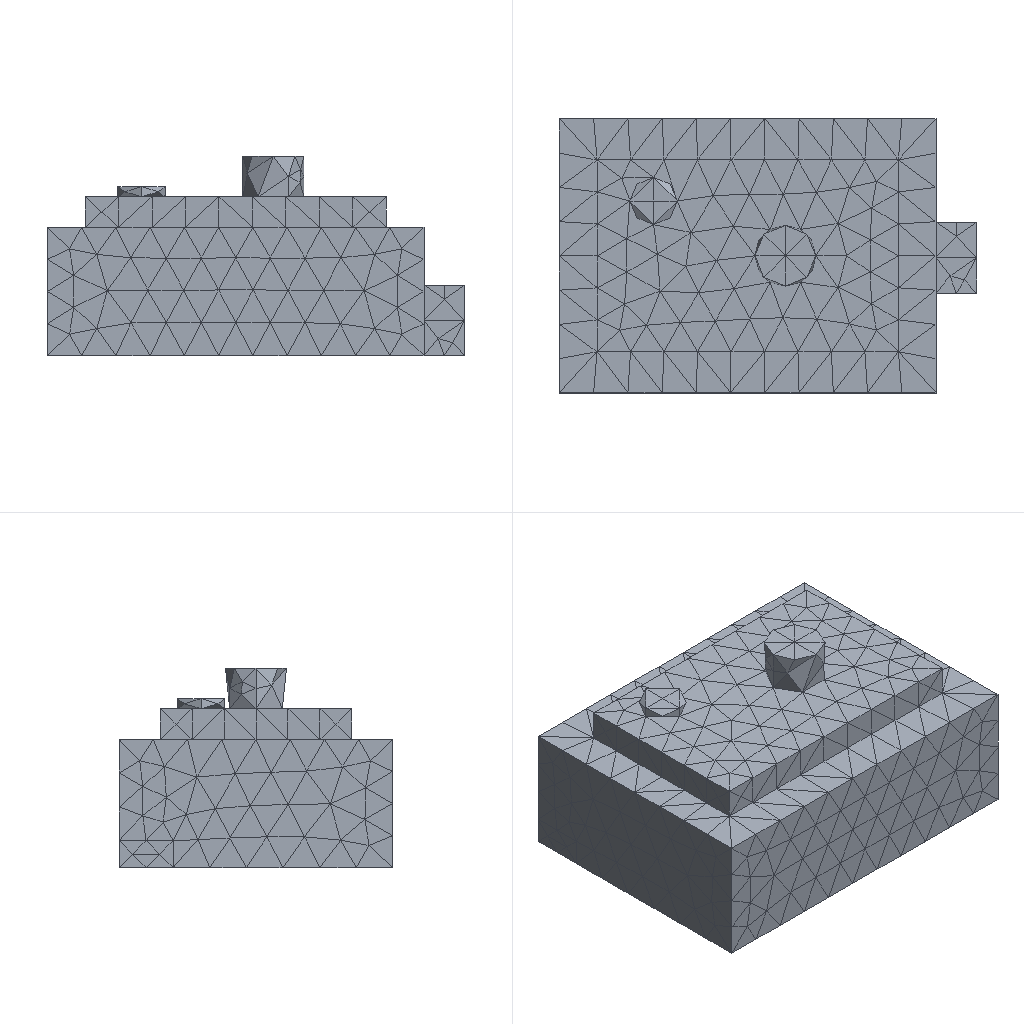Simulation study | ansys mapdl
Set-up summary:
category,name,step,type,value,unit,region
solver,ansys_mapdl
units,mm-N-s-tonne (MPa),,inferred,E=210000 density=
analysis,model,,static
mesh,nodes,,,5327
mesh,elements,,,3247
element_type,SOLID187,,,3247
material,mat 1,,E,210000
material,mat 1,,nu,0.3
load,,model,body load temp,,,all
load,,model,force,"1000 [dir=(0, 0, -1) n=175]",,node list
bc,,model,fixed,"[dofs=UX,UY,UZ n=5659]",,node list
Ansys APDL input file, long lists of numbers shortened:
/COM,ANSYS RELEASE 2026 R1           BUILD 26.1      UP20260202       09:09:40
/PREP7
/NOPR
/TITLE,2
ANTYPE, 0
*IF,_CDRDOFF,EQ,1,THEN     !if solid model was read in
_CDRDOFF=             !reset flag, numoffs already performed
*ELSE              !offset database for the following FE model
NUMOFF,NODE,     5327
NUMOFF,ELEM,     3247
NUMOFF,MAT ,        1
NUMOFF,TYPE,        1
*ENDIF
*SET,_RETURN ,  0.
*SET,_STATUS ,  0.
*SET,_UIQR   ,  175.
*SET,__FLOATPARAMETER__,  5327.
DOF,DELETE
ETBLOCK,        1,        1
(2i9,19a9)
        1      187        0        0        0        0        0        0        0        0        0        0        0        0        0        0        0        0        0        0        0
       -1
NBLOCK,6,SOLID,      5327,      5327
(3i9,6e21.13e3)
        1        0        0-3.9675000000000E+001 4.0500000000000E+001 8.0000000000000E+000
! (5326 more lines like these left out)
N,UNBL,LOC,       -1,
EBLOCK,19,SOLID,      3247,      3247
(19i10)
         1         1         1         1         0         0         0         0        10         0         1      1903      1904      1905      1906      2229      2230      2231      2232
! (6493 more lines like these left out)
        -1
MPTEMP,UNBL, 1, 1,  0.    ,
MPDATA,UNBL, 1,EX  ,       1, 1,  210000.000    ,
MPTEMP,UNBL, 1, 1,  0.    ,
MPDATA,UNBL, 1,NUXY,       1, 1, 0.3    ,
MPTEMP,UNBL, 1, 1,  0.    ,
MPDATA,UNBL, 1,PRXY,       1, 1, 0.3    ,
EXTOPT,ATTR,      0,      0,      0
EXTOPT,ESIZE,  0,  0.
EXTOPT,ACLEAR,      0
TREF,  0.
IRLF,  0
BFUNIF,TEMP,_TINY
ACEL,  0.    ,  0.    ,  0.
OMEGA,  0.    ,  0.    ,  0.
DOMEGA,  0.    ,  0.    ,  0.
CGLOC,  0.    ,  0.    ,  0.
CGOMEGA,  0.    ,  0.    ,  0.
DCGOMG,  0.    ,  0.    ,  0.
KUSE,     0
TIME,  0.
ALPHAD,  0.
BETAD,  0.
DMPRAT,  0.
DMPSTR,  0.
CRPLIM, 0.1    ,   0
CRPLIM,  0.    ,   1
NCNV,     0, 1.000000000E+12,     0,  0.    ,  0.
NEQIT,     0
ERESX,DEFA
DBLOCK,      5659
(i9,a6,2(pg16.9))
        1  UX    0.00000000      0.00000000
! (5658 more lines like these left out)
       -1
FBLOCK,       175
(i9,a6,2(pg16.9))
      919  FZ   -5.71428571      0.00000000
! (174 more lines like these left out)
       -1
/GO
FINISH
Results summary:
result,analysis_type_db,,,static,unstated
result,n_sets,,,1,unstated
result,load_steps[0].set,load_step=1,,1,unstated
result,load_steps[0].substep,load_step=1,,1,unstated
result,load_steps[0].time,load_step=1,,1,unstated
result,load_steps[0].freq,load_step=1,,1,unstated
result,load_steps[0].max_usum,load_step=1,,0.0002959,unstated
result,load_steps[0].max_seqv,load_step=1,,6.047,unstated
result,load_steps[0].reaction_sum.FX,load_step=1,,1.20141e-12,unstated
result,load_steps[0].reaction_sum.FY,load_step=1,,-2.70747e-11,unstated
result,load_steps[0].reaction_sum.FZ,load_step=1,,1000,unstated
result,load_steps[0].reaction_sum.MX,load_step=1,,0,unstated
result,load_steps[0].reaction_sum.MY,load_step=1,,0,unstated
result,load_steps[0].reaction_sum.MZ,load_step=1,,0,unstated
result,convergence,,,results present for all listed sets,unstated